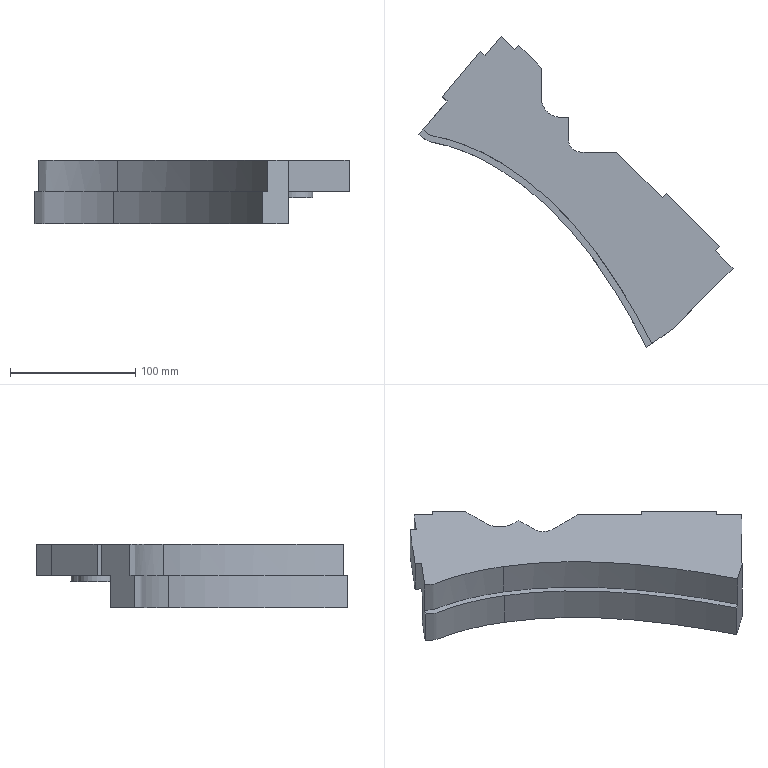Part | NX | features solid 2 | 1 solid | 42 faces | box 250.76 x 248.023 x 51 mm | volume 655863 mm3 | plane 28 | cylinder 7 | spline 7 | commonest cylinder face diameters 30 x6 20 x1